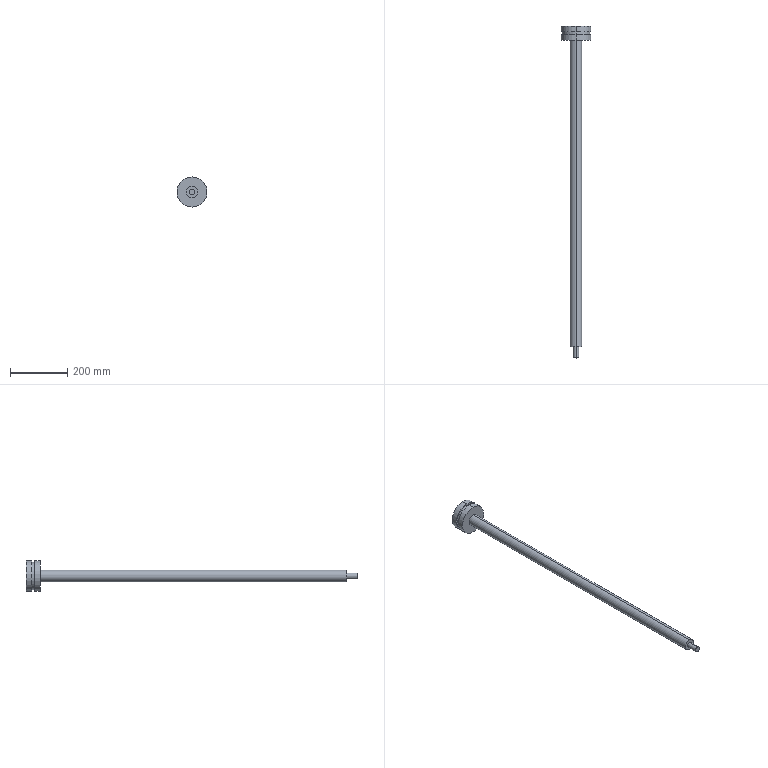Part | SolidWorks | features BaseBody 1 | 1 solid | 16 faces | box 105 x 1158 x 105 mm | volume 1771898 mm3 | cylinder 10 | plane 6 | commonest cylinder face diameters 105 x4 20 x2 40 x2 95 x2
STEP:
#1=CARTESIAN_POINT('',(0.,1068.,-20.));
#2=VERTEX_POINT('',#1);
#3=CARTESIAN_POINT('',(0.,1068.,20.));
#4=VERTEX_POINT('',#3);
#5=CARTESIAN_POINT('',(0.,1068.,0.));
#6=DIRECTION('',(0.,-1.,0.));
#7=DIRECTION('',(0.,0.,-1.));
#8=AXIS2_PLACEMENT_3D('',#5,#6,#7);
#9=CIRCLE('',#8,20.);
#10=EDGE_CURVE('',#2,#4,#9,.T.);
#11=ORIENTED_EDGE('',*,*,#10,.T.);
#12=CARTESIAN_POINT('',(0.,0.,20.));
#13=VERTEX_POINT('',#12);
#14=CARTESIAN_POINT('',(0.,1068.,20.));
#15=DIRECTION('',(0.,-1.,0.));
#16=VECTOR('',#15,1000.);
#17=LINE('',#14,#16);
#18=EDGE_CURVE('',#4,#13,#17,.T.);
#19=ORIENTED_EDGE('',*,*,#18,.T.);
#20=CARTESIAN_POINT('',(0.,0.,-20.));
#21=VERTEX_POINT('',#20);
#22=CARTESIAN_POINT('',(0.,0.,0.));
#23=DIRECTION('',(0.,1.,0.));
#24=DIRECTION('',(0.,0.,-1.));
#25=AXIS2_PLACEMENT_3D('',#22,#23,#24);
#26=CIRCLE('',#25,20.);
#27=EDGE_CURVE('',#13,#21,#26,.T.);
#28=ORIENTED_EDGE('',*,*,#27,.T.);
#29=CARTESIAN_POINT('',(0.,1068.,-20.));
#30=DIRECTION('',(0.,-1.,0.));
#31=VECTOR('',#30,1000.);
#32=LINE('',#29,#31);
#33=EDGE_CURVE('',#2,#21,#32,.T.);
#34=ORIENTED_EDGE('',*,*,#33,.F.);
#35=EDGE_LOOP('',(#11,#19,#28,#34));
#36=FACE_OUTER_BOUND('',#35,.T.);
#37=CARTESIAN_POINT('',(0.,1068.,0.));
#38=DIRECTION('',(0.,-1.,0.));
#39=DIRECTION('',(0.,0.,-1.));
#40=AXIS2_PLACEMENT_3D('',#37,#38,#39);
#41=CYLINDRICAL_SURFACE('',#40,20.);
#42=ADVANCED_FACE('',(#36),#41,.T.);
#43=CARTESIAN_POINT('',(0.,-40.,10.));
#44=VERTEX_POINT('',#43);
#45=CARTESIAN_POINT('',(0.,-40.,-10.));
#46=VERTEX_POINT('',#45);
#47=CARTESIAN_POINT('',(0.,-40.,0.));
#48=DIRECTION('',(0.,1.,0.));
#49=DIRECTION('',(0.,0.,1.));
#50=AXIS2_PLACEMENT_3D('',#47,#48,#49);
#51=CIRCLE('',#50,10.);
#52=EDGE_CURVE('',#44,#46,#51,.T.);
#53=ORIENTED_EDGE('',*,*,#52,.T.);
#54=CARTESIAN_POINT('',(0.,0.,-10.));
#55=VERTEX_POINT('',#54);
#56=CARTESIAN_POINT('',(0.,-40.,-10.));
#57=DIRECTION('',(0.,1.,0.));
#58=VECTOR('',#57,1000.);
#59=LINE('',#56,#58);
#60=EDGE_CURVE('',#46,#55,#59,.T.);
#61=ORIENTED_EDGE('',*,*,#60,.T.);
#62=CARTESIAN_POINT('',(0.,0.,10.));
#63=VERTEX_POINT('',#62);
#64=CARTESIAN_POINT('',(0.,0.,0.));
#65=DIRECTION('',(0.,-1.,0.));
#66=DIRECTION('',(0.,0.,1.));
#67=AXIS2_PLACEMENT_3D('',#64,#65,#66);
#68=CIRCLE('',#67,10.);
#69=EDGE_CURVE('',#55,#63,#68,.T.);
#70=ORIENTED_EDGE('',*,*,#69,.T.);
#71=CARTESIAN_POINT('',(0.,-40.,10.));
#72=DIRECTION('',(0.,1.,0.));
#73=VECTOR('',#72,1000.);
#74=LINE('',#71,#73);
#75=EDGE_CURVE('',#44,#63,#74,.T.);
#76=ORIENTED_EDGE('',*,*,#75,.F.);
#77=EDGE_LOOP('',(#53,#61,#70,#76));
#78=FACE_OUTER_BOUND('',#77,.T.);
#79=CARTESIAN_POINT('',(0.,-40.,0.));
#80=DIRECTION('',(0.,1.,0.));
#81=DIRECTION('',(0.,0.,1.));
#82=AXIS2_PLACEMENT_3D('',#79,#80,#81);
#83=CYLINDRICAL_SURFACE('',#82,10.);
#84=ADVANCED_FACE('',(#78),#83,.T.);
#85=CARTESIAN_POINT('',(0.,1088.,-52.5));
#86=VERTEX_POINT('',#85);
#87=CARTESIAN_POINT('',(0.,1088.,52.5));
#88=VERTEX_POINT('',#87);
#89=CARTESIAN_POINT('',(0.,1088.,0.));
#90=DIRECTION('',(0.,-1.,0.));
#91=DIRECTION('',(0.,0.,-1.));
#92=AXIS2_PLACEMENT_3D('',#89,#90,#91);
#93=CIRCLE('',#92,52.5);
#94=EDGE_CURVE('',#86,#88,#93,.T.);
#95=ORIENTED_EDGE('',*,*,#94,.T.);
#96=CARTESIAN_POINT('',(0.,1068.,52.5));
#97=VERTEX_POINT('',#96);
#98=CARTESIAN_POINT('',(0.,1088.,52.5));
#99=DIRECTION('',(0.,-1.,0.));
#100=VECTOR('',#99,1000.);
#101=LINE('',#98,#100);
#102=EDGE_CURVE('',#88,#97,#101,.T.);
#103=ORIENTED_EDGE('',*,*,#102,.T.);
#104=CARTESIAN_POINT('',(0.,1068.,-52.5));
#105=VERTEX_POINT('',#104);
#106=CARTESIAN_POINT('',(0.,1068.,0.));
#107=DIRECTION('',(0.,1.,0.));
#108=DIRECTION('',(0.,0.,-1.));
#109=AXIS2_PLACEMENT_3D('',#106,#107,#108);
#110=CIRCLE('',#109,52.5);
#111=EDGE_CURVE('',#97,#105,#110,.T.);
#112=ORIENTED_EDGE('',*,*,#111,.T.);
#113=CARTESIAN_POINT('',(0.,1088.,-52.5));
#114=DIRECTION('',(0.,-1.,0.));
#115=VECTOR('',#114,1000.);
#116=LINE('',#113,#115);
#117=EDGE_CURVE('',#86,#105,#116,.T.);
#118=ORIENTED_EDGE('',*,*,#117,.F.);
#119=EDGE_LOOP('',(#95,#103,#112,#118));
#120=FACE_OUTER_BOUND('',#119,.T.);
#121=CARTESIAN_POINT('',(0.,1088.,0.));
#122=DIRECTION('',(0.,-1.,0.));
#123=DIRECTION('',(0.,0.,-1.));
#124=AXIS2_PLACEMENT_3D('',#121,#122,#123);
#125=CYLINDRICAL_SURFACE('',#124,52.5);
#126=ADVANCED_FACE('',(#120),#125,.T.);
#127=CARTESIAN_POINT('',(0.,1098.,-47.5));
#128=VERTEX_POINT('',#127);
#129=CARTESIAN_POINT('',(0.,1098.,47.5));
#130=VERTEX_POINT('',#129);
#131=CARTESIAN_POINT('',(0.,1098.,0.));
#132=DIRECTION('',(0.,-1.,0.));
#133=DIRECTION('',(0.,0.,-1.));
#134=AXIS2_PLACEMENT_3D('',#131,#132,#133);
#135=CIRCLE('',#134,47.5);
#136=EDGE_CURVE('',#128,#130,#135,.T.);
#137=ORIENTED_EDGE('',*,*,#136,.T.);
#138=CARTESIAN_POINT('',(0.,1088.,47.5));
#139=VERTEX_POINT('',#138);
#140=CARTESIAN_POINT('',(0.,1098.,47.5));
#141=DIRECTION('',(0.,-1.,0.));
#142=VECTOR('',#141,1000.);
#143=LINE('',#140,#142);
#144=EDGE_CURVE('',#130,#139,#143,.T.);
#145=ORIENTED_EDGE('',*,*,#144,.T.);
#146=CARTESIAN_POINT('',(0.,1088.,-47.5));
#147=VERTEX_POINT('',#146);
#148=CARTESIAN_POINT('',(0.,1088.,0.));
#149=DIRECTION('',(0.,-1.,0.));
#150=DIRECTION('',(0.,0.,-1.));
#151=AXIS2_PLACEMENT_3D('',#148,#149,#150);
#152=CIRCLE('',#151,47.5);
#153=EDGE_CURVE('',#147,#139,#152,.T.);
#154=ORIENTED_EDGE('',*,*,#153,.F.);
#155=CARTESIAN_POINT('',(0.,1098.,-47.5));
#156=DIRECTION('',(0.,-1.,0.));
#157=VECTOR('',#156,1000.);
#158=LINE('',#155,#157);
#159=EDGE_CURVE('',#128,#147,#158,.T.);
#160=ORIENTED_EDGE('',*,*,#159,.F.);
#161=EDGE_LOOP('',(#137,#145,#154,#160));
#162=FACE_OUTER_BOUND('',#161,.T.);
#163=CARTESIAN_POINT('',(0.,1098.,0.));
#164=DIRECTION('',(0.,-1.,0.));
#165=DIRECTION('',(0.,0.,-1.));
#166=AXIS2_PLACEMENT_3D('',#163,#164,#165);
#167=CYLINDRICAL_SURFACE('',#166,47.5);
#168=ADVANCED_FACE('',(#162),#167,.T.);
#169=CARTESIAN_POINT('',(0.,1118.,-52.5));
#170=VERTEX_POINT('',#169);
#171=CARTESIAN_POINT('',(0.,1118.,52.5));
#172=VERTEX_POINT('',#171);
#173=CARTESIAN_POINT('',(0.,1118.,0.));
#174=DIRECTION('',(0.,-1.,0.));
#175=DIRECTION('',(0.,0.,-1.));
#176=AXIS2_PLACEMENT_3D('',#173,#174,#175);
#177=CIRCLE('',#176,52.5);
#178=EDGE_CURVE('',#170,#172,#177,.T.);
#179=ORIENTED_EDGE('',*,*,#178,.T.);
#180=CARTESIAN_POINT('',(0.,1098.,52.5));
#181=VERTEX_POINT('',#180);
#182=CARTESIAN_POINT('',(0.,1118.,52.5));
#183=DIRECTION('',(0.,-1.,0.));
#184=VECTOR('',#183,1000.);
#185=LINE('',#182,#184);
#186=EDGE_CURVE('',#172,#181,#185,.T.);
#187=ORIENTED_EDGE('',*,*,#186,.T.);
#188=CARTESIAN_POINT('',(0.,1098.,-52.5));
#189=VERTEX_POINT('',#188);
#190=CARTESIAN_POINT('',(0.,1098.,0.));
#191=DIRECTION('',(0.,1.,0.));
#192=DIRECTION('',(0.,0.,-1.));
#193=AXIS2_PLACEMENT_3D('',#190,#191,#192);
#194=CIRCLE('',#193,52.5);
#195=EDGE_CURVE('',#181,#189,#194,.T.);
#196=ORIENTED_EDGE('',*,*,#195,.T.);
#197=CARTESIAN_POINT('',(0.,1118.,-52.5));
#198=DIRECTION('',(0.,-1.,0.));
#199=VECTOR('',#198,1000.);
#200=LINE('',#197,#199);
#201=EDGE_CURVE('',#170,#189,#200,.T.);
#202=ORIENTED_EDGE('',*,*,#201,.F.);
#203=EDGE_LOOP('',(#179,#187,#196,#202));
#204=FACE_OUTER_BOUND('',#203,.T.);
#205=CARTESIAN_POINT('',(0.,1118.,0.));
#206=DIRECTION('',(0.,-1.,0.));
#207=DIRECTION('',(0.,0.,-1.));
#208=AXIS2_PLACEMENT_3D('',#205,#206,#207);
#209=CYLINDRICAL_SURFACE('',#208,52.5);
#210=ADVANCED_FACE('',(#204),#209,.T.);
#211=ORIENTED_EDGE('',*,*,#18,.F.);
#212=CARTESIAN_POINT('',(0.,1068.,0.));
#213=DIRECTION('',(0.,-1.,0.));
#214=DIRECTION('',(0.,0.,-1.));
#215=AXIS2_PLACEMENT_3D('',#212,#213,#214);
#216=CIRCLE('',#215,20.);
#217=EDGE_CURVE('',#4,#2,#216,.T.);
#218=ORIENTED_EDGE('',*,*,#217,.T.);
#219=ORIENTED_EDGE('',*,*,#33,.T.);
#220=CARTESIAN_POINT('',(0.,0.,0.));
#221=DIRECTION('',(0.,1.,0.));
#222=DIRECTION('',(0.,0.,-1.));
#223=AXIS2_PLACEMENT_3D('',#220,#221,#222);
#224=CIRCLE('',#223,20.);
#225=EDGE_CURVE('',#21,#13,#224,.T.);
#226=ORIENTED_EDGE('',*,*,#225,.T.);
#227=EDGE_LOOP('',(#211,#218,#219,#226));
#228=FACE_OUTER_BOUND('',#227,.T.);
#229=CARTESIAN_POINT('',(0.,1068.,0.));
#230=DIRECTION('',(0.,-1.,0.));
#231=DIRECTION('',(0.,0.,-1.));
#232=AXIS2_PLACEMENT_3D('',#229,#230,#231);
#233=CYLINDRICAL_SURFACE('',#232,20.);
#234=ADVANCED_FACE('',(#228),#233,.T.);
#235=ORIENTED_EDGE('',*,*,#225,.F.);
#236=ORIENTED_EDGE('',*,*,#27,.F.);
#237=EDGE_LOOP('',(#235,#236));
#238=FACE_OUTER_BOUND('',#237,.T.);
#239=CARTESIAN_POINT('',(0.,0.,0.));
#240=DIRECTION('',(0.,-1.,0.));
#241=DIRECTION('',(0.,0.,1.));
#242=AXIS2_PLACEMENT_3D('',#239,#240,#241);
#243=CIRCLE('',#242,10.);
#244=EDGE_CURVE('',#63,#55,#243,.T.);
#245=ORIENTED_EDGE('',*,*,#244,.F.);
#246=ORIENTED_EDGE('',*,*,#69,.F.);
#247=EDGE_LOOP('',(#245,#246));
#248=FACE_BOUND('',#247,.T.);
#249=CARTESIAN_POINT('',(0.,0.,0.));
#250=DIRECTION('',(0.,1.,0.));
#251=DIRECTION('',(0.,0.,1.));
#252=AXIS2_PLACEMENT_3D('',#249,#250,#251);
#253=PLANE('',#252);
#254=ADVANCED_FACE('',(#238,#248),#253,.F.);
#255=CARTESIAN_POINT('',(0.,1068.,0.));
#256=DIRECTION('',(0.,1.,0.));
#257=DIRECTION('',(0.,0.,-1.));
#258=AXIS2_PLACEMENT_3D('',#255,#256,#257);
#259=CIRCLE('',#258,52.5);
#260=EDGE_CURVE('',#105,#97,#259,.T.);
#261=ORIENTED_EDGE('',*,*,#260,.F.);
#262=ORIENTED_EDGE('',*,*,#111,.F.);
#263=EDGE_LOOP('',(#261,#262));
#264=FACE_OUTER_BOUND('',#263,.T.);
#265=ORIENTED_EDGE('',*,*,#10,.F.);
#266=ORIENTED_EDGE('',*,*,#217,.F.);
#267=EDGE_LOOP('',(#265,#266));
#268=FACE_BOUND('',#267,.T.);
#269=CARTESIAN_POINT('',(0.,1068.,0.));
#270=DIRECTION('',(0.,1.,0.));
#271=DIRECTION('',(0.,0.,1.));
#272=AXIS2_PLACEMENT_3D('',#269,#270,#271);
#273=PLANE('',#272);
#274=ADVANCED_FACE('',(#264,#268),#273,.F.);
#275=ORIENTED_EDGE('',*,*,#60,.F.);
#276=CARTESIAN_POINT('',(0.,-40.,0.));
#277=DIRECTION('',(0.,1.,0.));
#278=DIRECTION('',(0.,0.,1.));
#279=AXIS2_PLACEMENT_3D('',#276,#277,#278);
#280=CIRCLE('',#279,10.);
#281=EDGE_CURVE('',#46,#44,#280,.T.);
#282=ORIENTED_EDGE('',*,*,#281,.T.);
#283=ORIENTED_EDGE('',*,*,#75,.T.);
#284=ORIENTED_EDGE('',*,*,#244,.T.);
#285=EDGE_LOOP('',(#275,#282,#283,#284));
#286=FACE_OUTER_BOUND('',#285,.T.);
#287=CARTESIAN_POINT('',(0.,-40.,0.));
#288=DIRECTION('',(0.,1.,0.));
#289=DIRECTION('',(0.,0.,1.));
#290=AXIS2_PLACEMENT_3D('',#287,#288,#289);
#291=CYLINDRICAL_SURFACE('',#290,10.);
#292=ADVANCED_FACE('',(#286),#291,.T.);
#293=ORIENTED_EDGE('',*,*,#102,.F.);
#294=CARTESIAN_POINT('',(0.,1088.,0.));
#295=DIRECTION('',(0.,-1.,0.));
#296=DIRECTION('',(0.,0.,-1.));
#297=AXIS2_PLACEMENT_3D('',#294,#295,#296);
#298=CIRCLE('',#297,52.5);
#299=EDGE_CURVE('',#88,#86,#298,.T.);
#300=ORIENTED_EDGE('',*,*,#299,.T.);
#301=ORIENTED_EDGE('',*,*,#117,.T.);
#302=ORIENTED_EDGE('',*,*,#260,.T.);
#303=EDGE_LOOP('',(#293,#300,#301,#302));
#304=FACE_OUTER_BOUND('',#303,.T.);
#305=CARTESIAN_POINT('',(0.,1088.,0.));
#306=DIRECTION('',(0.,-1.,0.));
#307=DIRECTION('',(0.,0.,-1.));
#308=AXIS2_PLACEMENT_3D('',#305,#306,#307);
#309=CYLINDRICAL_SURFACE('',#308,52.5);
#310=ADVANCED_FACE('',(#304),#309,.T.);
#311=ORIENTED_EDGE('',*,*,#52,.F.);
#312=ORIENTED_EDGE('',*,*,#281,.F.);
#313=EDGE_LOOP('',(#311,#312));
#314=FACE_OUTER_BOUND('',#313,.T.);
#315=CARTESIAN_POINT('',(0.,-40.,0.));
#316=DIRECTION('',(0.,-1.,0.));
#317=DIRECTION('',(0.,0.,-1.));
#318=AXIS2_PLACEMENT_3D('',#315,#316,#317);
#319=PLANE('',#318);
#320=ADVANCED_FACE('',(#314),#319,.T.);
#321=ORIENTED_EDGE('',*,*,#94,.F.);
#322=ORIENTED_EDGE('',*,*,#299,.F.);
#323=EDGE_LOOP('',(#321,#322));
#324=FACE_OUTER_BOUND('',#323,.T.);
#325=ORIENTED_EDGE('',*,*,#153,.T.);
#326=CARTESIAN_POINT('',(0.,1088.,0.));
#327=DIRECTION('',(0.,-1.,0.));
#328=DIRECTION('',(0.,0.,-1.));
#329=AXIS2_PLACEMENT_3D('',#326,#327,#328);
#330=CIRCLE('',#329,47.5);
#331=EDGE_CURVE('',#139,#147,#330,.T.);
#332=ORIENTED_EDGE('',*,*,#331,.T.);
#333=EDGE_LOOP('',(#325,#332));
#334=FACE_BOUND('',#333,.T.);
#335=CARTESIAN_POINT('',(0.,1088.,0.));
#336=DIRECTION('',(0.,1.,0.));
#337=DIRECTION('',(0.,0.,1.));
#338=AXIS2_PLACEMENT_3D('',#335,#336,#337);
#339=PLANE('',#338);
#340=ADVANCED_FACE('',(#324,#334),#339,.T.);
#341=ORIENTED_EDGE('',*,*,#144,.F.);
#342=CARTESIAN_POINT('',(0.,1098.,0.));
#343=DIRECTION('',(0.,-1.,0.));
#344=DIRECTION('',(0.,0.,-1.));
#345=AXIS2_PLACEMENT_3D('',#342,#343,#344);
#346=CIRCLE('',#345,47.5);
#347=EDGE_CURVE('',#130,#128,#346,.T.);
#348=ORIENTED_EDGE('',*,*,#347,.T.);
#349=ORIENTED_EDGE('',*,*,#159,.T.);
#350=ORIENTED_EDGE('',*,*,#331,.F.);
#351=EDGE_LOOP('',(#341,#348,#349,#350));
#352=FACE_OUTER_BOUND('',#351,.T.);
#353=CARTESIAN_POINT('',(0.,1098.,0.));
#354=DIRECTION('',(0.,-1.,0.));
#355=DIRECTION('',(0.,0.,-1.));
#356=AXIS2_PLACEMENT_3D('',#353,#354,#355);
#357=CYLINDRICAL_SURFACE('',#356,47.5);
#358=ADVANCED_FACE('',(#352),#357,.T.);
#359=CARTESIAN_POINT('',(0.,1098.,0.));
#360=DIRECTION('',(0.,1.,0.));
#361=DIRECTION('',(0.,0.,-1.));
#362=AXIS2_PLACEMENT_3D('',#359,#360,#361);
#363=CIRCLE('',#362,52.5);
#364=EDGE_CURVE('',#189,#181,#363,.T.);
#365=ORIENTED_EDGE('',*,*,#364,.F.);
#366=ORIENTED_EDGE('',*,*,#195,.F.);
#367=EDGE_LOOP('',(#365,#366));
#368=FACE_OUTER_BOUND('',#367,.T.);
#369=ORIENTED_EDGE('',*,*,#136,.F.);
#370=ORIENTED_EDGE('',*,*,#347,.F.);
#371=EDGE_LOOP('',(#369,#370));
#372=FACE_BOUND('',#371,.T.);
#373=CARTESIAN_POINT('',(0.,1098.,0.));
#374=DIRECTION('',(0.,1.,0.));
#375=DIRECTION('',(0.,0.,1.));
#376=AXIS2_PLACEMENT_3D('',#373,#374,#375);
#377=PLANE('',#376);
#378=ADVANCED_FACE('',(#368,#372),#377,.F.);
#379=ORIENTED_EDGE('',*,*,#186,.F.);
#380=CARTESIAN_POINT('',(0.,1118.,0.));
#381=DIRECTION('',(0.,-1.,0.));
#382=DIRECTION('',(0.,0.,-1.));
#383=AXIS2_PLACEMENT_3D('',#380,#381,#382);
#384=CIRCLE('',#383,52.5);
#385=EDGE_CURVE('',#172,#170,#384,.T.);
#386=ORIENTED_EDGE('',*,*,#385,.T.);
#387=ORIENTED_EDGE('',*,*,#201,.T.);
#388=ORIENTED_EDGE('',*,*,#364,.T.);
#389=EDGE_LOOP('',(#379,#386,#387,#388));
#390=FACE_OUTER_BOUND('',#389,.T.);
#391=CARTESIAN_POINT('',(0.,1118.,0.));
#392=DIRECTION('',(0.,-1.,0.));
#393=DIRECTION('',(0.,0.,-1.));
#394=AXIS2_PLACEMENT_3D('',#391,#392,#393);
#395=CYLINDRICAL_SURFACE('',#394,52.5);
#396=ADVANCED_FACE('',(#390),#395,.T.);
#397=ORIENTED_EDGE('',*,*,#178,.F.);
#398=ORIENTED_EDGE('',*,*,#385,.F.);
#399=EDGE_LOOP('',(#397,#398));
#400=FACE_OUTER_BOUND('',#399,.T.);
#401=CARTESIAN_POINT('',(0.,1118.,0.));
#402=DIRECTION('',(0.,1.,0.));
#403=DIRECTION('',(0.,0.,1.));
#404=AXIS2_PLACEMENT_3D('',#401,#402,#403);
#405=PLANE('',#404);
#406=ADVANCED_FACE('',(#400),#405,.T.);
#407=CLOSED_SHELL('',(#42,#84,#126,#168,#210,#234,#254,#274,#292,#310,#320,#340,#358,#378,#396,#406));
#408=MANIFOLD_SOLID_BREP('',#407);
#409=CARTESIAN_POINT('',(0.,0.,0.));
#410=DIRECTION('',(0.,0.,1.));
#411=DIRECTION('',(1.,0.,0.));
#412=AXIS2_PLACEMENT_3D('',#409,#410,#411);
#413=(LENGTH_UNIT()NAMED_UNIT(*)SI_UNIT(.MILLI.,.METRE.));
#414=UNCERTAINTY_MEASURE_WITH_UNIT(LENGTH_MEASURE(0.00001),#413,'','');
#415=(NAMED_UNIT(*)PLANE_ANGLE_UNIT()SI_UNIT($,.RADIAN.));
#416=(NAMED_UNIT(*)SI_UNIT($,.STERADIAN.)SOLID_ANGLE_UNIT());
#417=(GEOMETRIC_REPRESENTATION_CONTEXT(3)GLOBAL_UNCERTAINTY_ASSIGNED_CONTEXT((#414))GLOBAL_UNIT_ASSIGNED_CONTEXT((#413,#415,#416))REPRESENTATION_CONTEXT('',''));
#418=ADVANCED_BREP_SHAPE_REPRESENTATION('',(#408,#412),#417);